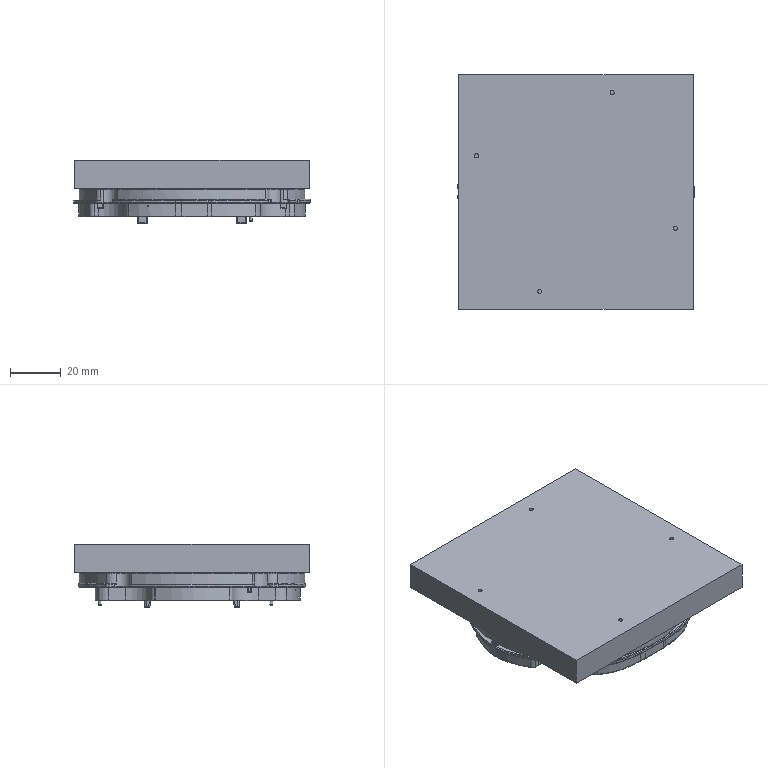Part | 2 solids | 774 faces | box 92.935 x 92.1 x 24.829 mm | volume 135568 mm3 | cylinder 270 | plane 251 | torus 178 | spline 47 | sphere 18 | cone 10 | commonest cylinder face diameters 0.6 x91 4 x18 1 x16 10 x14 1.6 x12 5 x10